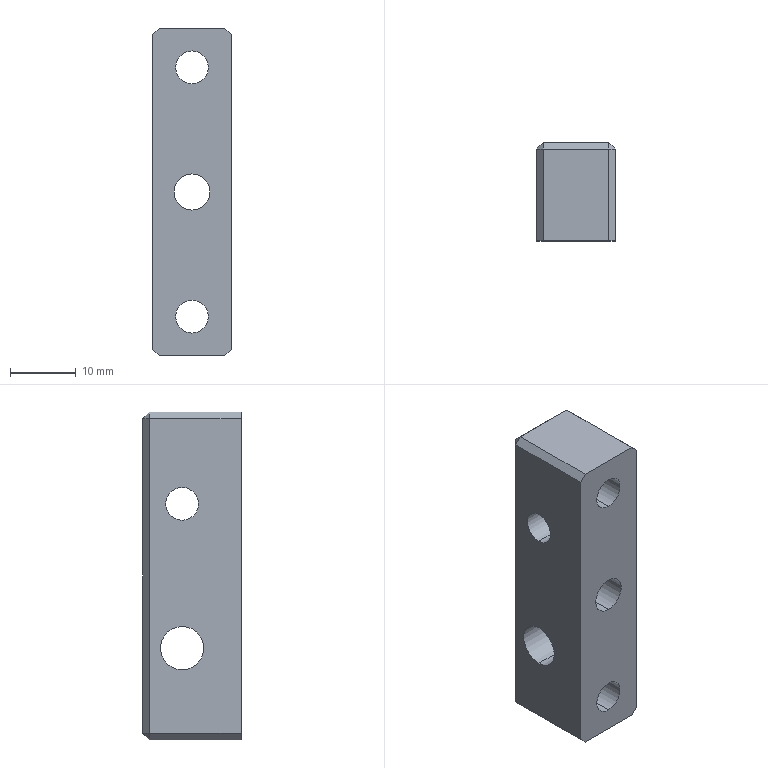Part | SolidWorks | features HoleWzd 3, Chamfer 1, Extrusion 1, ICE 1 | 1 solid | 32 faces | box 12 x 15 x 50 mm | volume 6990 mm3 | plane 20 | cylinder 12 | commonest cylinder face diameters 5 x6 5.5 x2 6.6 x2 10 x2
STEP:
#1=CARTESIAN_POINT('',(0.,9.,-11.5));
#2=VERTEX_POINT('',#1);
#3=CARTESIAN_POINT('',(0.,9.,-16.5));
#4=VERTEX_POINT('',#3);
#5=CARTESIAN_POINT('',(0.,9.,-14.));
#6=DIRECTION('',(1.,0.,0.));
#7=DIRECTION('',(0.,0.,-1.));
#8=AXIS2_PLACEMENT_3D('',#5,#6,#7);
#9=CIRCLE('',#8,2.5);
#10=EDGE_CURVE('',#2,#4,#9,.T.);
#11=ORIENTED_EDGE('',*,*,#10,.F.);
#12=CARTESIAN_POINT('',(12.,9.,-11.5));
#13=VERTEX_POINT('',#12);
#14=CARTESIAN_POINT('',(12.,9.,-11.5));
#15=DIRECTION('',(1.,0.,0.));
#16=VECTOR('',#15,1000.);
#17=LINE('',#14,#16);
#18=EDGE_CURVE('',#2,#13,#17,.T.);
#19=ORIENTED_EDGE('',*,*,#18,.T.);
#20=CARTESIAN_POINT('',(12.,9.,-16.5));
#21=VERTEX_POINT('',#20);
#22=CARTESIAN_POINT('',(12.,9.,-14.));
#23=DIRECTION('',(1.,0.,0.));
#24=DIRECTION('',(0.,0.,-1.));
#25=AXIS2_PLACEMENT_3D('',#22,#23,#24);
#26=CIRCLE('',#25,2.5);
#27=EDGE_CURVE('',#13,#21,#26,.T.);
#28=ORIENTED_EDGE('',*,*,#27,.T.);
#29=CARTESIAN_POINT('',(12.,9.,-16.5));
#30=DIRECTION('',(1.,0.,0.));
#31=VECTOR('',#30,1000.);
#32=LINE('',#29,#31);
#33=EDGE_CURVE('',#4,#21,#32,.T.);
#34=ORIENTED_EDGE('',*,*,#33,.F.);
#35=EDGE_LOOP('',(#11,#19,#28,#34));
#36=FACE_OUTER_BOUND('',#35,.T.);
#37=CARTESIAN_POINT('',(12.,9.,-14.));
#38=DIRECTION('',(1.,0.,0.));
#39=DIRECTION('',(0.,0.,-1.));
#40=AXIS2_PLACEMENT_3D('',#37,#38,#39);
#41=CYLINDRICAL_SURFACE('',#40,2.5);
#42=ADVANCED_FACE('',(#36),#41,.F.);
#43=CARTESIAN_POINT('',(0.,9.,-32.7));
#44=VERTEX_POINT('',#43);
#45=CARTESIAN_POINT('',(0.,9.,-39.3));
#46=VERTEX_POINT('',#45);
#47=CARTESIAN_POINT('',(0.,9.,-36.));
#48=DIRECTION('',(1.,0.,0.));
#49=DIRECTION('',(0.,0.,-1.));
#50=AXIS2_PLACEMENT_3D('',#47,#48,#49);
#51=CIRCLE('',#50,3.3);
#52=EDGE_CURVE('',#44,#46,#51,.T.);
#53=ORIENTED_EDGE('',*,*,#52,.F.);
#54=CARTESIAN_POINT('',(12.,9.,-32.7));
#55=VERTEX_POINT('',#54);
#56=CARTESIAN_POINT('',(12.,9.,-32.7));
#57=DIRECTION('',(1.,0.,0.));
#58=VECTOR('',#57,1000.);
#59=LINE('',#56,#58);
#60=EDGE_CURVE('',#44,#55,#59,.T.);
#61=ORIENTED_EDGE('',*,*,#60,.T.);
#62=CARTESIAN_POINT('',(12.,9.,-39.3));
#63=VERTEX_POINT('',#62);
#64=CARTESIAN_POINT('',(12.,9.,-36.));
#65=DIRECTION('',(1.,0.,0.));
#66=DIRECTION('',(0.,0.,-1.));
#67=AXIS2_PLACEMENT_3D('',#64,#65,#66);
#68=CIRCLE('',#67,3.3);
#69=EDGE_CURVE('',#55,#63,#68,.T.);
#70=ORIENTED_EDGE('',*,*,#69,.T.);
#71=CARTESIAN_POINT('',(12.,9.,-39.3));
#72=DIRECTION('',(1.,0.,0.));
#73=VECTOR('',#72,1000.);
#74=LINE('',#71,#73);
#75=EDGE_CURVE('',#46,#63,#74,.T.);
#76=ORIENTED_EDGE('',*,*,#75,.F.);
#77=EDGE_LOOP('',(#53,#61,#70,#76));
#78=FACE_OUTER_BOUND('',#77,.T.);
#79=CARTESIAN_POINT('',(12.,9.,-36.));
#80=DIRECTION('',(1.,0.,0.));
#81=DIRECTION('',(0.,0.,-1.));
#82=AXIS2_PLACEMENT_3D('',#79,#80,#81);
#83=CYLINDRICAL_SURFACE('',#82,3.3);
#84=ADVANCED_FACE('',(#78),#83,.F.);
#85=CARTESIAN_POINT('',(6.,9.,-30.));
#86=VERTEX_POINT('',#85);
#87=CARTESIAN_POINT('',(6.,9.,-20.));
#88=VERTEX_POINT('',#87);
#89=CARTESIAN_POINT('',(6.,9.,-25.));
#90=DIRECTION('',(0.,1.,0.));
#91=DIRECTION('',(0.,0.,1.));
#92=AXIS2_PLACEMENT_3D('',#89,#90,#91);
#93=CIRCLE('',#92,5.);
#94=EDGE_CURVE('',#86,#88,#93,.T.);
#95=ORIENTED_EDGE('',*,*,#94,.F.);
#96=CARTESIAN_POINT('',(6.,15.,-30.));
#97=VERTEX_POINT('',#96);
#98=CARTESIAN_POINT('',(6.,15.,-30.));
#99=DIRECTION('',(0.,1.,0.));
#100=VECTOR('',#99,1000.);
#101=LINE('',#98,#100);
#102=EDGE_CURVE('',#86,#97,#101,.T.);
#103=ORIENTED_EDGE('',*,*,#102,.T.);
#104=CARTESIAN_POINT('',(1.,15.,-25.));
#105=VERTEX_POINT('',#104);
#106=CARTESIAN_POINT('',(6.,15.,-25.));
#107=DIRECTION('',(0.,1.,0.));
#108=DIRECTION('',(0.,0.,1.));
#109=AXIS2_PLACEMENT_3D('',#106,#107,#108);
#110=CIRCLE('',#109,5.);
#111=EDGE_CURVE('',#97,#105,#110,.T.);
#112=ORIENTED_EDGE('',*,*,#111,.T.);
#113=CARTESIAN_POINT('',(6.,15.,-20.));
#114=VERTEX_POINT('',#113);
#115=CARTESIAN_POINT('',(6.,15.,-25.));
#116=DIRECTION('',(0.,1.,0.));
#117=DIRECTION('',(0.,0.,1.));
#118=AXIS2_PLACEMENT_3D('',#115,#116,#117);
#119=CIRCLE('',#118,5.);
#120=EDGE_CURVE('',#105,#114,#119,.T.);
#121=ORIENTED_EDGE('',*,*,#120,.T.);
#122=CARTESIAN_POINT('',(6.,15.,-20.));
#123=DIRECTION('',(0.,1.,0.));
#124=VECTOR('',#123,1000.);
#125=LINE('',#122,#124);
#126=EDGE_CURVE('',#88,#114,#125,.T.);
#127=ORIENTED_EDGE('',*,*,#126,.F.);
#128=EDGE_LOOP('',(#95,#103,#112,#121,#127));
#129=FACE_OUTER_BOUND('',#128,.T.);
#130=CARTESIAN_POINT('',(6.,15.,-25.));
#131=DIRECTION('',(0.,1.,0.));
#132=DIRECTION('',(0.,0.,1.));
#133=AXIS2_PLACEMENT_3D('',#130,#131,#132);
#134=CYLINDRICAL_SURFACE('',#133,5.);
#135=ADVANCED_FACE('',(#129),#134,.F.);
#136=CARTESIAN_POINT('',(6.,0.,-27.75));
#137=VERTEX_POINT('',#136);
#138=CARTESIAN_POINT('',(6.,0.,-22.25));
#139=VERTEX_POINT('',#138);
#140=CARTESIAN_POINT('',(6.,0.,-25.));
#141=DIRECTION('',(0.,1.,0.));
#142=DIRECTION('',(0.,0.,1.));
#143=AXIS2_PLACEMENT_3D('',#140,#141,#142);
#144=CIRCLE('',#143,2.75);
#145=EDGE_CURVE('',#137,#139,#144,.T.);
#146=ORIENTED_EDGE('',*,*,#145,.F.);
#147=CARTESIAN_POINT('',(6.,9.,-27.75));
#148=VERTEX_POINT('',#147);
#149=CARTESIAN_POINT('',(6.,15.,-27.75));
#150=DIRECTION('',(0.,1.,0.));
#151=VECTOR('',#150,1000.);
#152=LINE('',#149,#151);
#153=EDGE_CURVE('',#137,#148,#152,.T.);
#154=ORIENTED_EDGE('',*,*,#153,.T.);
#155=CARTESIAN_POINT('',(6.,9.,-22.25));
#156=VERTEX_POINT('',#155);
#157=CARTESIAN_POINT('',(6.,9.,-25.));
#158=DIRECTION('',(0.,1.,0.));
#159=DIRECTION('',(0.,0.,1.));
#160=AXIS2_PLACEMENT_3D('',#157,#158,#159);
#161=CIRCLE('',#160,2.75);
#162=EDGE_CURVE('',#148,#156,#161,.T.);
#163=ORIENTED_EDGE('',*,*,#162,.T.);
#164=CARTESIAN_POINT('',(6.,15.,-22.25));
#165=DIRECTION('',(0.,1.,0.));
#166=VECTOR('',#165,1000.);
#167=LINE('',#164,#166);
#168=EDGE_CURVE('',#139,#156,#167,.T.);
#169=ORIENTED_EDGE('',*,*,#168,.F.);
#170=EDGE_LOOP('',(#146,#154,#163,#169));
#171=FACE_OUTER_BOUND('',#170,.T.);
#172=CARTESIAN_POINT('',(6.,15.,-25.));
#173=DIRECTION('',(0.,1.,0.));
#174=DIRECTION('',(0.,0.,1.));
#175=AXIS2_PLACEMENT_3D('',#172,#173,#174);
#176=CYLINDRICAL_SURFACE('',#175,2.75);
#177=ADVANCED_FACE('',(#171),#176,.F.);
#178=CARTESIAN_POINT('',(6.,0.,-8.5));
#179=VERTEX_POINT('',#178);
#180=CARTESIAN_POINT('',(6.,0.,-3.5));
#181=VERTEX_POINT('',#180);
#182=CARTESIAN_POINT('',(6.,0.,-6.));
#183=DIRECTION('',(0.,1.,0.));
#184=DIRECTION('',(0.,0.,1.));
#185=AXIS2_PLACEMENT_3D('',#182,#183,#184);
#186=CIRCLE('',#185,2.5);
#187=EDGE_CURVE('',#179,#181,#186,.T.);
#188=ORIENTED_EDGE('',*,*,#187,.F.);
#189=CARTESIAN_POINT('',(6.,15.,-8.5));
#190=VERTEX_POINT('',#189);
#191=CARTESIAN_POINT('',(6.,0.,-8.5));
#192=DIRECTION('',(0.,1.,0.));
#193=VECTOR('',#192,1000.);
#194=LINE('',#191,#193);
#195=EDGE_CURVE('',#179,#190,#194,.T.);
#196=ORIENTED_EDGE('',*,*,#195,.T.);
#197=CARTESIAN_POINT('',(6.,15.,-3.5));
#198=VERTEX_POINT('',#197);
#199=CARTESIAN_POINT('',(6.,15.,-6.));
#200=DIRECTION('',(0.,1.,0.));
#201=DIRECTION('',(0.,0.,1.));
#202=AXIS2_PLACEMENT_3D('',#199,#200,#201);
#203=CIRCLE('',#202,2.5);
#204=EDGE_CURVE('',#190,#198,#203,.T.);
#205=ORIENTED_EDGE('',*,*,#204,.T.);
#206=CARTESIAN_POINT('',(6.,0.,-3.5));
#207=DIRECTION('',(0.,1.,0.));
#208=VECTOR('',#207,1000.);
#209=LINE('',#206,#208);
#210=EDGE_CURVE('',#181,#198,#209,.T.);
#211=ORIENTED_EDGE('',*,*,#210,.F.);
#212=EDGE_LOOP('',(#188,#196,#205,#211));
#213=FACE_OUTER_BOUND('',#212,.T.);
#214=CARTESIAN_POINT('',(6.,0.,-6.));
#215=DIRECTION('',(0.,1.,0.));
#216=DIRECTION('',(0.,0.,1.));
#217=AXIS2_PLACEMENT_3D('',#214,#215,#216);
#218=CYLINDRICAL_SURFACE('',#217,2.5);
#219=ADVANCED_FACE('',(#213),#218,.F.);
#220=CARTESIAN_POINT('',(6.,0.,-46.5));
#221=VERTEX_POINT('',#220);
#222=CARTESIAN_POINT('',(6.,0.,-41.5));
#223=VERTEX_POINT('',#222);
#224=CARTESIAN_POINT('',(6.,0.,-44.));
#225=DIRECTION('',(0.,1.,0.));
#226=DIRECTION('',(0.,0.,1.));
#227=AXIS2_PLACEMENT_3D('',#224,#225,#226);
#228=CIRCLE('',#227,2.5);
#229=EDGE_CURVE('',#221,#223,#228,.T.);
#230=ORIENTED_EDGE('',*,*,#229,.F.);
#231=CARTESIAN_POINT('',(6.,15.,-46.5));
#232=VERTEX_POINT('',#231);
#233=CARTESIAN_POINT('',(6.,0.,-46.5));
#234=DIRECTION('',(0.,1.,0.));
#235=VECTOR('',#234,1000.);
#236=LINE('',#233,#235);
#237=EDGE_CURVE('',#221,#232,#236,.T.);
#238=ORIENTED_EDGE('',*,*,#237,.T.);
#239=CARTESIAN_POINT('',(6.,15.,-41.5));
#240=VERTEX_POINT('',#239);
#241=CARTESIAN_POINT('',(6.,15.,-44.));
#242=DIRECTION('',(0.,1.,0.));
#243=DIRECTION('',(0.,0.,1.));
#244=AXIS2_PLACEMENT_3D('',#241,#242,#243);
#245=CIRCLE('',#244,2.5);
#246=EDGE_CURVE('',#232,#240,#245,.T.);
#247=ORIENTED_EDGE('',*,*,#246,.T.);
#248=CARTESIAN_POINT('',(6.,0.,-41.5));
#249=DIRECTION('',(0.,1.,0.));
#250=VECTOR('',#249,1000.);
#251=LINE('',#248,#250);
#252=EDGE_CURVE('',#223,#240,#251,.T.);
#253=ORIENTED_EDGE('',*,*,#252,.F.);
#254=EDGE_LOOP('',(#230,#238,#247,#253));
#255=FACE_OUTER_BOUND('',#254,.T.);
#256=CARTESIAN_POINT('',(6.,0.,-44.));
#257=DIRECTION('',(0.,1.,0.));
#258=DIRECTION('',(0.,0.,1.));
#259=AXIS2_PLACEMENT_3D('',#256,#257,#258);
#260=CYLINDRICAL_SURFACE('',#259,2.5);
#261=ADVANCED_FACE('',(#255),#260,.F.);
#262=CARTESIAN_POINT('',(6.,15.,-44.));
#263=DIRECTION('',(0.,1.,0.));
#264=DIRECTION('',(0.,0.,1.));
#265=AXIS2_PLACEMENT_3D('',#262,#263,#264);
#266=CIRCLE('',#265,2.5);
#267=EDGE_CURVE('',#240,#232,#266,.T.);
#268=ORIENTED_EDGE('',*,*,#267,.F.);
#269=ORIENTED_EDGE('',*,*,#246,.F.);
#270=EDGE_LOOP('',(#268,#269));
#271=FACE_BOUND('',#270,.T.);
#272=CARTESIAN_POINT('',(11.,15.,-25.));
#273=VERTEX_POINT('',#272);
#274=CARTESIAN_POINT('',(11.,15.,-49.));
#275=VERTEX_POINT('',#274);
#276=CARTESIAN_POINT('',(11.,15.,0.));
#277=DIRECTION('',(0.,0.,-1.));
#278=VECTOR('',#277,1000.);
#279=LINE('',#276,#278);
#280=EDGE_CURVE('',#273,#275,#279,.T.);
#281=ORIENTED_EDGE('',*,*,#280,.T.);
#282=CARTESIAN_POINT('',(1.,15.,-49.));
#283=VERTEX_POINT('',#282);
#284=CARTESIAN_POINT('',(0.,15.,-49.));
#285=DIRECTION('',(-1.,0.,0.));
#286=VECTOR('',#285,1000.);
#287=LINE('',#284,#286);
#288=EDGE_CURVE('',#275,#283,#287,.T.);
#289=ORIENTED_EDGE('',*,*,#288,.T.);
#290=CARTESIAN_POINT('',(1.,15.,0.));
#291=DIRECTION('',(0.,0.,1.));
#292=VECTOR('',#291,1000.);
#293=LINE('',#290,#292);
#294=EDGE_CURVE('',#283,#105,#293,.T.);
#295=ORIENTED_EDGE('',*,*,#294,.T.);
#296=ORIENTED_EDGE('',*,*,#111,.F.);
#297=CARTESIAN_POINT('',(6.,15.,-25.));
#298=DIRECTION('',(0.,1.,0.));
#299=DIRECTION('',(0.,0.,1.));
#300=AXIS2_PLACEMENT_3D('',#297,#298,#299);
#301=CIRCLE('',#300,5.);
#302=EDGE_CURVE('',#273,#97,#301,.T.);
#303=ORIENTED_EDGE('',*,*,#302,.F.);
#304=EDGE_LOOP('',(#281,#289,#295,#296,#303));
#305=FACE_OUTER_BOUND('',#304,.T.);
#306=CARTESIAN_POINT('',(0.,15.,0.));
#307=DIRECTION('',(0.,-1.,0.));
#308=DIRECTION('',(0.,0.,-1.));
#309=AXIS2_PLACEMENT_3D('',#306,#307,#308);
#310=PLANE('',#309);
#311=ADVANCED_FACE('',(#271,#305),#310,.F.);
#312=CARTESIAN_POINT('',(0.,9.,-14.));
#313=DIRECTION('',(1.,0.,0.));
#314=DIRECTION('',(0.,0.,-1.));
#315=AXIS2_PLACEMENT_3D('',#312,#313,#314);
#316=CIRCLE('',#315,2.5);
#317=EDGE_CURVE('',#4,#2,#316,.T.);
#318=ORIENTED_EDGE('',*,*,#317,.T.);
#319=ORIENTED_EDGE('',*,*,#10,.T.);
#320=EDGE_LOOP('',(#318,#319));
#321=FACE_BOUND('',#320,.T.);
#322=CARTESIAN_POINT('',(0.,9.,-36.));
#323=DIRECTION('',(1.,0.,0.));
#324=DIRECTION('',(0.,0.,-1.));
#325=AXIS2_PLACEMENT_3D('',#322,#323,#324);
#326=CIRCLE('',#325,3.3);
#327=EDGE_CURVE('',#46,#44,#326,.T.);
#328=ORIENTED_EDGE('',*,*,#327,.T.);
#329=ORIENTED_EDGE('',*,*,#52,.T.);
#330=EDGE_LOOP('',(#328,#329));
#331=FACE_BOUND('',#330,.T.);
#332=CARTESIAN_POINT('',(0.,14.,-1.));
#333=VERTEX_POINT('',#332);
#334=CARTESIAN_POINT('',(0.,14.,-49.));
#335=VERTEX_POINT('',#334);
#336=CARTESIAN_POINT('',(0.,14.,0.));
#337=DIRECTION('',(0.,0.,-1.));
#338=VECTOR('',#337,1000.);
#339=LINE('',#336,#338);
#340=EDGE_CURVE('',#333,#335,#339,.T.);
#341=ORIENTED_EDGE('',*,*,#340,.T.);
#342=CARTESIAN_POINT('',(0.,0.,-49.));
#343=VERTEX_POINT('',#342);
#344=CARTESIAN_POINT('',(0.,15.,-49.));
#345=DIRECTION('',(0.,-1.,0.));
#346=VECTOR('',#345,1000.);
#347=LINE('',#344,#346);
#348=EDGE_CURVE('',#335,#343,#347,.T.);
#349=ORIENTED_EDGE('',*,*,#348,.T.);
#350=CARTESIAN_POINT('',(0.,0.,-1.));
#351=VERTEX_POINT('',#350);
#352=CARTESIAN_POINT('',(0.,0.,0.));
#353=DIRECTION('',(0.,0.,1.));
#354=VECTOR('',#353,1000.);
#355=LINE('',#352,#354);
#356=EDGE_CURVE('',#343,#351,#355,.T.);
#357=ORIENTED_EDGE('',*,*,#356,.T.);
#358=CARTESIAN_POINT('',(0.,15.,-1.));
#359=DIRECTION('',(0.,1.,0.));
#360=VECTOR('',#359,1000.);
#361=LINE('',#358,#360);
#362=EDGE_CURVE('',#351,#333,#361,.T.);
#363=ORIENTED_EDGE('',*,*,#362,.T.);
#364=EDGE_LOOP('',(#341,#349,#357,#363));
#365=FACE_OUTER_BOUND('',#364,.T.);
#366=CARTESIAN_POINT('',(0.,15.,0.));
#367=DIRECTION('',(1.,0.,0.));
#368=DIRECTION('',(0.,0.,-1.));
#369=AXIS2_PLACEMENT_3D('',#366,#367,#368);
#370=PLANE('',#369);
#371=ADVANCED_FACE('',(#321,#331,#365),#370,.F.);
#372=CARTESIAN_POINT('',(11.,14.,0.));
#373=VERTEX_POINT('',#372);
#374=CARTESIAN_POINT('',(1.,14.,0.));
#375=VERTEX_POINT('',#374);
#376=CARTESIAN_POINT('',(0.,14.,0.));
#377=DIRECTION('',(-1.,0.,0.));
#378=VECTOR('',#377,1000.);
#379=LINE('',#376,#378);
#380=EDGE_CURVE('',#373,#375,#379,.T.);
#381=ORIENTED_EDGE('',*,*,#380,.T.);
#382=CARTESIAN_POINT('',(1.,0.,0.));
#383=VERTEX_POINT('',#382);
#384=CARTESIAN_POINT('',(1.,15.,0.));
#385=DIRECTION('',(0.,-1.,0.));
#386=VECTOR('',#385,1000.);
#387=LINE('',#384,#386);
#388=EDGE_CURVE('',#375,#383,#387,.T.);
#389=ORIENTED_EDGE('',*,*,#388,.T.);
#390=CARTESIAN_POINT('',(11.,0.,0.));
#391=VERTEX_POINT('',#390);
#392=CARTESIAN_POINT('',(0.,0.,0.));
#393=DIRECTION('',(1.,0.,0.));
#394=VECTOR('',#393,1000.);
#395=LINE('',#392,#394);
#396=EDGE_CURVE('',#383,#391,#395,.T.);
#397=ORIENTED_EDGE('',*,*,#396,.T.);
#398=CARTESIAN_POINT('',(11.,15.,0.));
#399=DIRECTION('',(0.,1.,0.));
#400=VECTOR('',#399,1000.);
#401=LINE('',#398,#400);
#402=EDGE_CURVE('',#391,#373,#401,.T.);
#403=ORIENTED_EDGE('',*,*,#402,.T.);
#404=EDGE_LOOP('',(#381,#389,#397,#403));
#405=FACE_OUTER_BOUND('',#404,.T.);
#406=CARTESIAN_POINT('',(0.,15.,0.));
#407=DIRECTION('',(0.,0.,-1.));
#408=DIRECTION('',(-1.,0.,0.));
#409=AXIS2_PLACEMENT_3D('',#406,#407,#408);
#410=PLANE('',#409);
#411=ADVANCED_FACE('',(#405),#410,.F.);
#412=CARTESIAN_POINT('',(12.,9.,-14.));
#413=DIRECTION('',(1.,0.,0.));
#414=DIRECTION('',(0.,0.,-1.));
#415=AXIS2_PLACEMENT_3D('',#412,#413,#414);
#416=CIRCLE('',#415,2.5);
#417=EDGE_CURVE('',#21,#13,#416,.T.);
#418=ORIENTED_EDGE('',*,*,#417,.F.);
#419=ORIENTED_EDGE('',*,*,#27,.F.);
#420=EDGE_LOOP('',(#418,#419));
#421=FACE_BOUND('',#420,.T.);
#422=CARTESIAN_POINT('',(12.,9.,-36.));
#423=DIRECTION('',(1.,0.,0.));
#424=DIRECTION('',(0.,0.,-1.));
#425=AXIS2_PLACEMENT_3D('',#422,#423,#424);
#426=CIRCLE('',#425,3.3);
#427=EDGE_CURVE('',#63,#55,#426,.T.);
#428=ORIENTED_EDGE('',*,*,#427,.F.);
#429=ORIENTED_EDGE('',*,*,#69,.F.);
#430=EDGE_LOOP('',(#428,#429));
#431=FACE_BOUND('',#430,.T.);
#432=CARTESIAN_POINT('',(12.,0.,-1.));
#433=VERTEX_POINT('',#432);
#434=CARTESIAN_POINT('',(12.,0.,-49.));
#435=VERTEX_POINT('',#434);
#436=CARTESIAN_POINT('',(12.,0.,0.));
#437=DIRECTION('',(0.,0.,-1.));
#438=VECTOR('',#437,1000.);
#439=LINE('',#436,#438);
#440=EDGE_CURVE('',#433,#435,#439,.T.);
#441=ORIENTED_EDGE('',*,*,#440,.T.);
#442=CARTESIAN_POINT('',(12.,14.,-49.));
#443=VERTEX_POINT('',#442);
#444=CARTESIAN_POINT('',(12.,15.,-49.));
#445=DIRECTION('',(0.,1.,0.));
#446=VECTOR('',#445,1000.);
#447=LINE('',#444,#446);
#448=EDGE_CURVE('',#435,#443,#447,.T.);
#449=ORIENTED_EDGE('',*,*,#448,.T.);
#450=CARTESIAN_POINT('',(12.,14.,-1.));
#451=VERTEX_POINT('',#450);
#452=CARTESIAN_POINT('',(12.,14.,0.));
#453=DIRECTION('',(0.,0.,1.));
#454=VECTOR('',#453,1000.);
#455=LINE('',#452,#454);
#456=EDGE_CURVE('',#443,#451,#455,.T.);
#457=ORIENTED_EDGE('',*,*,#456,.T.);
#458=CARTESIAN_POINT('',(12.,15.,-1.));
#459=DIRECTION('',(0.,-1.,0.));
#460=VECTOR('',#459,1000.);
#461=LINE('',#458,#460);
#462=EDGE_CURVE('',#451,#433,#461,.T.);
#463=ORIENTED_EDGE('',*,*,#462,.T.);
#464=EDGE_LOOP('',(#441,#449,#457,#463));
#465=FACE_OUTER_BOUND('',#464,.T.);
#466=CARTESIAN_POINT('',(12.,15.,0.));
#467=DIRECTION('',(-1.,0.,0.));
#468=DIRECTION('',(0.,0.,1.));
#469=AXIS2_PLACEMENT_3D('',#466,#467,#468);
#470=PLANE('',#469);
#471=ADVANCED_FACE('',(#421,#431,#465),#470,.F.);
#472=CARTESIAN_POINT('',(11.,0.,-50.));
#473=VERTEX_POINT('',#472);
#474=CARTESIAN_POINT('',(1.,0.,-50.));
#475=VERTEX_POINT('',#474);
#476=CARTESIAN_POINT('',(0.,0.,-50.));
#477=DIRECTION('',(-1.,0.,0.));
#478=VECTOR('',#477,1000.);
#479=LINE('',#476,#478);
#480=EDGE_CURVE('',#473,#475,#479,.T.);
#481=ORIENTED_EDGE('',*,*,#480,.T.);
#482=CARTESIAN_POINT('',(1.,14.,-50.));
#483=VERTEX_POINT('',#482);
#484=CARTESIAN_POINT('',(1.,15.,-50.));
#485=DIRECTION('',(0.,1.,0.));
#486=VECTOR('',#485,1000.);
#487=LINE('',#484,#486);
#488=EDGE_CURVE('',#475,#483,#487,.T.);
#489=ORIENTED_EDGE('',*,*,#488,.T.);
#490=CARTESIAN_POINT('',(11.,14.,-50.));
#491=VERTEX_POINT('',#490);
#492=CARTESIAN_POINT('',(0.,14.,-50.));
#493=DIRECTION('',(1.,0.,0.));
#494=VECTOR('',#493,1000.);
#495=LINE('',#492,#494);
#496=EDGE_CURVE('',#483,#491,#495,.T.);
#497=ORIENTED_EDGE('',*,*,#496,.T.);
#498=CARTESIAN_POINT('',(11.,15.,-50.));
#499=DIRECTION('',(0.,-1.,0.));
#500=VECTOR('',#499,1000.);
#501=LINE('',#498,#500);
#502=EDGE_CURVE('',#491,#473,#501,.T.);
#503=ORIENTED_EDGE('',*,*,#502,.T.);
#504=EDGE_LOOP('',(#481,#489,#497,#503));
#505=FACE_OUTER_BOUND('',#504,.T.);
#506=CARTESIAN_POINT('',(0.,15.,-50.));
#507=DIRECTION('',(0.,0.,1.));
#508=DIRECTION('',(1.,0.,0.));
#509=AXIS2_PLACEMENT_3D('',#506,#507,#508);
#510=PLANE('',#509);
#511=ADVANCED_FACE('',(#505),#510,.F.);
#512=ORIENTED_EDGE('',*,*,#120,.F.);
#513=CARTESIAN_POINT('',(1.,15.,-1.));
#514=VERTEX_POINT('',#513);
#515=CARTESIAN_POINT('',(1.,15.,0.));
#516=DIRECTION('',(0.,0.,1.));
#517=VECTOR('',#516,1000.);
#518=LINE('',#515,#517);
#519=EDGE_CURVE('',#105,#514,#518,.T.);
#520=ORIENTED_EDGE('',*,*,#519,.T.);
#521=CARTESIAN_POINT('',(11.,15.,-1.));
#522=VERTEX_POINT('',#521);
#523=CARTESIAN_POINT('',(0.,15.,-1.));
#524=DIRECTION('',(1.,0.,0.));
#525=VECTOR('',#524,1000.);
#526=LINE('',#523,#525);
#527=EDGE_CURVE('',#514,#522,#526,.T.);
#528=ORIENTED_EDGE('',*,*,#527,.T.);
#529=CARTESIAN_POINT('',(11.,15.,0.));
#530=DIRECTION('',(0.,0.,-1.));
#531=VECTOR('',#530,1000.);
#532=LINE('',#529,#531);
#533=EDGE_CURVE('',#522,#273,#532,.T.);
#534=ORIENTED_EDGE('',*,*,#533,.T.);
#535=CARTESIAN_POINT('',(6.,15.,-25.));
#536=DIRECTION('',(0.,1.,0.));
#537=DIRECTION('',(0.,0.,1.));
#538=AXIS2_PLACEMENT_3D('',#535,#536,#537);
#539=CIRCLE('',#538,5.);
#540=EDGE_CURVE('',#114,#273,#539,.T.);
#541=ORIENTED_EDGE('',*,*,#540,.F.);
#542=EDGE_LOOP('',(#512,#520,#528,#534,#541));
#543=FACE_OUTER_BOUND('',#542,.T.);
#544=CARTESIAN_POINT('',(6.,15.,-6.));
#545=DIRECTION('',(0.,1.,0.));
#546=DIRECTION('',(0.,0.,1.));
#547=AXIS2_PLACEMENT_3D('',#544,#545,#546);
#548=CIRCLE('',#547,2.5);
#549=EDGE_CURVE('',#198,#190,#548,.T.);
#550=ORIENTED_EDGE('',*,*,#549,.F.);
#551=ORIENTED_EDGE('',*,*,#204,.F.);
#552=EDGE_LOOP('',(#550,#551));
#553=FACE_BOUND('',#552,.T.);
#554=CARTESIAN_POINT('',(0.,15.,0.));
#555=DIRECTION('',(0.,-1.,0.));
#556=DIRECTION('',(0.,0.,-1.));
#557=AXIS2_PLACEMENT_3D('',#554,#555,#556);
#558=PLANE('',#557);
#559=ADVANCED_FACE('',(#543,#553),#558,.F.);
#560=CARTESIAN_POINT('',(6.,0.,-25.));
#561=DIRECTION('',(0.,1.,0.));
#562=DIRECTION('',(0.,0.,1.));
#563=AXIS2_PLACEMENT_3D('',#560,#561,#562);
#564=CIRCLE('',#563,2.75);
#565=EDGE_CURVE('',#139,#137,#564,.T.);
#566=ORIENTED_EDGE('',*,*,#565,.T.);
#567=ORIENTED_EDGE('',*,*,#145,.T.);
#568=EDGE_LOOP('',(#566,#567));
#569=FACE_BOUND('',#568,.T.);
#570=CARTESIAN_POINT('',(6.,0.,-6.));
#571=DIRECTION('',(0.,1.,0.));
#572=DIRECTION('',(0.,0.,1.));
#573=AXIS2_PLACEMENT_3D('',#570,#571,#572);
#574=CIRCLE('',#573,2.5);
#575=EDGE_CURVE('',#181,#179,#574,.T.);
#576=ORIENTED_EDGE('',*,*,#575,.T.);
#577=ORIENTED_EDGE('',*,*,#187,.T.);
#578=EDGE_LOOP('',(#576,#577));
#579=FACE_BOUND('',#578,.T.);
#580=CARTESIAN_POINT('',(6.,0.,-44.));
#581=DIRECTION('',(0.,1.,0.));
#582=DIRECTION('',(0.,0.,1.));
#583=AXIS2_PLACEMENT_3D('',#580,#581,#582);
#584=CIRCLE('',#583,2.5);
#585=EDGE_CURVE('',#223,#221,#584,.T.);
#586=ORIENTED_EDGE('',*,*,#585,.T.);
#587=ORIENTED_EDGE('',*,*,#229,.T.);
#588=EDGE_LOOP('',(#586,#587));
#589=FACE_BOUND('',#588,.T.);
#590=ORIENTED_EDGE('',*,*,#356,.F.);
#591=CARTESIAN_POINT('',(-24.5,0.,-24.5));
#592=DIRECTION('',(0.7071,0.,-0.7071));
#593=VECTOR('',#592,1000.);
#594=LINE('',#591,#593);
#595=EDGE_CURVE('',#343,#475,#594,.T.);
#596=ORIENTED_EDGE('',*,*,#595,.T.);
#597=ORIENTED_EDGE('',*,*,#480,.F.);
#598=CARTESIAN_POINT('',(30.5,0.,-30.5));
#599=DIRECTION('',(0.7071,0.,0.7071));
#600=VECTOR('',#599,1000.);
#601=LINE('',#598,#600);
#602=EDGE_CURVE('',#473,#435,#601,.T.);
#603=ORIENTED_EDGE('',*,*,#602,.T.);
#604=ORIENTED_EDGE('',*,*,#440,.F.);
#605=CARTESIAN_POINT('',(5.5,0.,5.5));
#606=DIRECTION('',(-0.7071,0.,0.7071));
#607=VECTOR('',#606,1000.);
#608=LINE('',#605,#607);
#609=EDGE_CURVE('',#433,#391,#608,.T.);
#610=ORIENTED_EDGE('',*,*,#609,.T.);
#611=ORIENTED_EDGE('',*,*,#396,.F.);
#612=CARTESIAN_POINT('',(0.5,0.,-0.5));
#613=DIRECTION('',(-0.7071,0.,-0.7071));
#614=VECTOR('',#613,1000.);
#615=LINE('',#612,#614);
#616=EDGE_CURVE('',#383,#351,#615,.T.);
#617=ORIENTED_EDGE('',*,*,#616,.T.);
#618=EDGE_LOOP('',(#590,#596,#597,#603,#604,#610,#611,#617));
#619=FACE_OUTER_BOUND('',#618,.T.);
#620=CARTESIAN_POINT('',(0.,0.,0.));
#621=DIRECTION('',(0.,-1.,0.));
#622=DIRECTION('',(0.,0.,-1.));
#623=AXIS2_PLACEMENT_3D('',#620,#621,#622);
#624=PLANE('',#623);
#625=ADVANCED_FACE('',(#569,#579,#589,#619),#624,.T.);
#626=ORIENTED_EDGE('',*,*,#237,.F.);
#627=ORIENTED_EDGE('',*,*,#585,.F.);
#628=ORIENTED_EDGE('',*,*,#252,.T.);
#629=ORIENTED_EDGE('',*,*,#267,.T.);
#630=EDGE_LOOP('',(#626,#627,#628,#629));
#631=FACE_OUTER_BOUND('',#630,.T.);
#632=CARTESIAN_POINT('',(6.,0.,-44.));
#633=DIRECTION('',(0.,1.,0.));
#634=DIRECTION('',(0.,0.,1.));
#635=AXIS2_PLACEMENT_3D('',#632,#633,#634);
#636=CYLINDRICAL_SURFACE('',#635,2.5);
#637=ADVANCED_FACE('',(#631),#636,.F.);
#638=ORIENTED_EDGE('',*,*,#195,.F.);
#639=ORIENTED_EDGE('',*,*,#575,.F.);
#640=ORIENTED_EDGE('',*,*,#210,.T.);
#641=ORIENTED_EDGE('',*,*,#549,.T.);
#642=EDGE_LOOP('',(#638,#639,#640,#641));
#643=FACE_OUTER_BOUND('',#642,.T.);
#644=CARTESIAN_POINT('',(6.,0.,-6.));
#645=DIRECTION('',(0.,1.,0.));
#646=DIRECTION('',(0.,0.,1.));
#647=AXIS2_PLACEMENT_3D('',#644,#645,#646);
#648=CYLINDRICAL_SURFACE('',#647,2.5);
#649=ADVANCED_FACE('',(#643),#648,.F.);
#650=ORIENTED_EDGE('',*,*,#153,.F.);
#651=ORIENTED_EDGE('',*,*,#565,.F.);
#652=ORIENTED_EDGE('',*,*,#168,.T.);
#653=CARTESIAN_POINT('',(6.,9.,-25.));
#654=DIRECTION('',(0.,1.,0.));
#655=DIRECTION('',(0.,0.,1.));
#656=AXIS2_PLACEMENT_3D('',#653,#654,#655);
#657=CIRCLE('',#656,2.75);
#658=EDGE_CURVE('',#156,#148,#657,.T.);
#659=ORIENTED_EDGE('',*,*,#658,.T.);
#660=EDGE_LOOP('',(#650,#651,#652,#659));
#661=FACE_OUTER_BOUND('',#660,.T.);
#662=CARTESIAN_POINT('',(6.,15.,-25.));
#663=DIRECTION('',(0.,1.,0.));
#664=DIRECTION('',(0.,0.,1.));
#665=AXIS2_PLACEMENT_3D('',#662,#663,#664);
#666=CYLINDRICAL_SURFACE('',#665,2.75);
#667=ADVANCED_FACE('',(#661),#666,.F.);
#668=ORIENTED_EDGE('',*,*,#658,.F.);
#669=ORIENTED_EDGE('',*,*,#162,.F.);
#670=EDGE_LOOP('',(#668,#669));
#671=FACE_BOUND('',#670,.T.);
#672=CARTESIAN_POINT('',(6.,9.,-25.));
#673=DIRECTION('',(0.,1.,0.));
#674=DIRECTION('',(0.,0.,1.));
#675=AXIS2_PLACEMENT_3D('',#672,#673,#674);
#676=CIRCLE('',#675,5.);
#677=EDGE_CURVE('',#88,#86,#676,.T.);
#678=ORIENTED_EDGE('',*,*,#677,.T.);
#679=ORIENTED_EDGE('',*,*,#94,.T.);
#680=EDGE_LOOP('',(#678,#679));
#681=FACE_OUTER_BOUND('',#680,.T.);
#682=CARTESIAN_POINT('',(8.75,9.,-25.));
#683=DIRECTION('',(0.,-1.,0.));
#684=DIRECTION('',(0.,0.,-1.));
#685=AXIS2_PLACEMENT_3D('',#682,#683,#684);
#686=PLANE('',#685);
#687=ADVANCED_FACE('',(#671,#681),#686,.F.);
#688=ORIENTED_EDGE('',*,*,#102,.F.);
#689=ORIENTED_EDGE('',*,*,#677,.F.);
#690=ORIENTED_EDGE('',*,*,#126,.T.);
#691=ORIENTED_EDGE('',*,*,#540,.T.);
#692=ORIENTED_EDGE('',*,*,#302,.T.);
#693=EDGE_LOOP('',(#688,#689,#690,#691,#692));
#694=FACE_OUTER_BOUND('',#693,.T.);
#695=CARTESIAN_POINT('',(6.,15.,-25.));
#696=DIRECTION('',(0.,1.,0.));
#697=DIRECTION('',(0.,0.,1.));
#698=AXIS2_PLACEMENT_3D('',#695,#696,#697);
#699=CYLINDRICAL_SURFACE('',#698,5.);
#700=ADVANCED_FACE('',(#694),#699,.F.);
#701=ORIENTED_EDGE('',*,*,#60,.F.);
#702=ORIENTED_EDGE('',*,*,#327,.F.);
#703=ORIENTED_EDGE('',*,*,#75,.T.);
#704=ORIENTED_EDGE('',*,*,#427,.T.);
#705=EDGE_LOOP('',(#701,#702,#703,#704));
#706=FACE_OUTER_BOUND('',#705,.T.);
#707=CARTESIAN_POINT('',(12.,9.,-36.));
#708=DIRECTION('',(1.,0.,0.));
#709=DIRECTION('',(0.,0.,-1.));
#710=AXIS2_PLACEMENT_3D('',#707,#708,#709);
#711=CYLINDRICAL_SURFACE('',#710,3.3);
#712=ADVANCED_FACE('',(#706),#711,.F.);
#713=ORIENTED_EDGE('',*,*,#18,.F.);
#714=ORIENTED_EDGE('',*,*,#317,.F.);
#715=ORIENTED_EDGE('',*,*,#33,.T.);
#716=ORIENTED_EDGE('',*,*,#417,.T.);
#717=EDGE_LOOP('',(#713,#714,#715,#716));
#718=FACE_OUTER_BOUND('',#717,.T.);
#719=CARTESIAN_POINT('',(12.,9.,-14.));
#720=DIRECTION('',(1.,0.,0.));
#721=DIRECTION('',(0.,0.,-1.));
#722=AXIS2_PLACEMENT_3D('',#719,#720,#721);
#723=CYLINDRICAL_SURFACE('',#722,2.5);
#724=ADVANCED_FACE('',(#718),#723,.F.);
#725=ORIENTED_EDGE('',*,*,#602,.F.);
#726=ORIENTED_EDGE('',*,*,#502,.F.);
#727=CARTESIAN_POINT('',(12.,14.,-49.));
#728=DIRECTION('',(-0.7071,0.,-0.7071));
#729=VECTOR('',#728,1000.);
#730=LINE('',#727,#729);
#731=EDGE_CURVE('',#443,#491,#730,.T.);
#732=ORIENTED_EDGE('',*,*,#731,.F.);
#733=ORIENTED_EDGE('',*,*,#448,.F.);
#734=EDGE_LOOP('',(#725,#726,#732,#733));
#735=FACE_OUTER_BOUND('',#734,.T.);
#736=CARTESIAN_POINT('',(11.,15.,-50.));
#737=DIRECTION('',(-0.7071,0.,0.7071));
#738=DIRECTION('',(0.,-1.,0.));
#739=AXIS2_PLACEMENT_3D('',#736,#737,#738);
#740=PLANE('',#739);
#741=ADVANCED_FACE('',(#735),#740,.F.);
#742=CARTESIAN_POINT('',(12.,14.,-1.));
#743=DIRECTION('',(-0.7071,0.7071,0.));
#744=VECTOR('',#743,1000.);
#745=LINE('',#742,#744);
#746=EDGE_CURVE('',#451,#522,#745,.T.);
#747=ORIENTED_EDGE('',*,*,#746,.F.);
#748=ORIENTED_EDGE('',*,*,#456,.F.);
#749=CARTESIAN_POINT('',(12.,14.,-49.));
#750=DIRECTION('',(0.7071,-0.7071,0.));
#751=VECTOR('',#750,1000.);
#752=LINE('',#749,#751);
#753=EDGE_CURVE('',#275,#443,#752,.T.);
#754=ORIENTED_EDGE('',*,*,#753,.F.);
#755=ORIENTED_EDGE('',*,*,#280,.F.);
#756=ORIENTED_EDGE('',*,*,#533,.F.);
#757=EDGE_LOOP('',(#747,#748,#754,#755,#756));
#758=FACE_OUTER_BOUND('',#757,.T.);
#759=CARTESIAN_POINT('',(11.,15.,0.));
#760=DIRECTION('',(-0.7071,-0.7071,0.));
#761=DIRECTION('',(0.,0.,-1.));
#762=AXIS2_PLACEMENT_3D('',#759,#760,#761);
#763=PLANE('',#762);
#764=ADVANCED_FACE('',(#758),#763,.F.);
#765=ORIENTED_EDGE('',*,*,#609,.F.);
#766=ORIENTED_EDGE('',*,*,#462,.F.);
#767=CARTESIAN_POINT('',(12.,14.,-1.));
#768=DIRECTION('',(0.7071,0.,-0.7071));
#769=VECTOR('',#768,1000.);
#770=LINE('',#767,#769);
#771=EDGE_CURVE('',#373,#451,#770,.T.);
#772=ORIENTED_EDGE('',*,*,#771,.F.);
#773=ORIENTED_EDGE('',*,*,#402,.F.);
#774=EDGE_LOOP('',(#765,#766,#772,#773));
#775=FACE_OUTER_BOUND('',#774,.T.);
#776=CARTESIAN_POINT('',(12.,15.,-1.));
#777=DIRECTION('',(-0.7071,0.,-0.7071));
#778=DIRECTION('',(0.,-1.,0.));
#779=AXIS2_PLACEMENT_3D('',#776,#777,#778);
#780=PLANE('',#779);
#781=ADVANCED_FACE('',(#775),#780,.F.);
#782=ORIENTED_EDGE('',*,*,#753,.T.);
#783=ORIENTED_EDGE('',*,*,#731,.T.);
#784=CARTESIAN_POINT('',(11.,14.5,-49.5));
#785=DIRECTION('',(0.,-0.7071,-0.7071));
#786=VECTOR('',#785,1000.);
#787=LINE('',#784,#786);
#788=EDGE_CURVE('',#275,#491,#787,.T.);
#789=ORIENTED_EDGE('',*,*,#788,.F.);
#790=EDGE_LOOP('',(#782,#783,#789));
#791=FACE_OUTER_BOUND('',#790,.T.);
#792=CARTESIAN_POINT('',(12.,14.,-49.));
#793=DIRECTION('',(0.5774,0.5774,-0.5774));
#794=DIRECTION('',(-0.7071,0.,-0.7071));
#795=AXIS2_PLACEMENT_3D('',#792,#793,#794);
#796=PLANE('',#795);
#797=ADVANCED_FACE('',(#791),#796,.T.);
#798=ORIENTED_EDGE('',*,*,#771,.T.);
#799=ORIENTED_EDGE('',*,*,#746,.T.);
#800=CARTESIAN_POINT('',(11.,14.5,-0.5));
#801=DIRECTION('',(0.,0.7071,-0.7071));
#802=VECTOR('',#801,1000.);
#803=LINE('',#800,#802);
#804=EDGE_CURVE('',#373,#522,#803,.T.);
#805=ORIENTED_EDGE('',*,*,#804,.F.);
#806=EDGE_LOOP('',(#798,#799,#805));
#807=FACE_OUTER_BOUND('',#806,.T.);
#808=CARTESIAN_POINT('',(12.,14.,-1.));
#809=DIRECTION('',(0.5774,0.5774,0.5774));
#810=DIRECTION('',(0.7071,0.,-0.7071));
#811=AXIS2_PLACEMENT_3D('',#808,#809,#810);
#812=PLANE('',#811);
#813=ADVANCED_FACE('',(#807),#812,.T.);
#814=ORIENTED_EDGE('',*,*,#595,.F.);
#815=ORIENTED_EDGE('',*,*,#348,.F.);
#816=CARTESIAN_POINT('',(0.,14.,-49.));
#817=DIRECTION('',(-0.7071,0.,0.7071));
#818=VECTOR('',#817,1000.);
#819=LINE('',#816,#818);
#820=EDGE_CURVE('',#483,#335,#819,.T.);
#821=ORIENTED_EDGE('',*,*,#820,.F.);
#822=ORIENTED_EDGE('',*,*,#488,.F.);
#823=EDGE_LOOP('',(#814,#815,#821,#822));
#824=FACE_OUTER_BOUND('',#823,.T.);
#825=CARTESIAN_POINT('',(0.,15.,-49.));
#826=DIRECTION('',(0.7071,0.,0.7071));
#827=DIRECTION('',(0.,-1.,0.));
#828=AXIS2_PLACEMENT_3D('',#825,#826,#827);
#829=PLANE('',#828);
#830=ADVANCED_FACE('',(#824),#829,.F.);
#831=ORIENTED_EDGE('',*,*,#788,.T.);
#832=ORIENTED_EDGE('',*,*,#496,.F.);
#833=CARTESIAN_POINT('',(1.,14.5,-49.5));
#834=DIRECTION('',(0.,-0.7071,-0.7071));
#835=VECTOR('',#834,1000.);
#836=LINE('',#833,#835);
#837=EDGE_CURVE('',#283,#483,#836,.T.);
#838=ORIENTED_EDGE('',*,*,#837,.F.);
#839=ORIENTED_EDGE('',*,*,#288,.F.);
#840=EDGE_LOOP('',(#831,#832,#838,#839));
#841=FACE_OUTER_BOUND('',#840,.T.);
#842=CARTESIAN_POINT('',(0.,15.,-49.));
#843=DIRECTION('',(0.,-0.7071,0.7071));
#844=DIRECTION('',(-1.,0.,0.));
#845=AXIS2_PLACEMENT_3D('',#842,#843,#844);
#846=PLANE('',#845);
#847=ADVANCED_FACE('',(#841),#846,.F.);
#848=ORIENTED_EDGE('',*,*,#804,.T.);
#849=ORIENTED_EDGE('',*,*,#527,.F.);
#850=CARTESIAN_POINT('',(1.,15.,-1.));
#851=DIRECTION('',(0.,0.7071,-0.7071));
#852=VECTOR('',#851,1000.);
#853=LINE('',#850,#852);
#854=EDGE_CURVE('',#375,#514,#853,.T.);
#855=ORIENTED_EDGE('',*,*,#854,.F.);
#856=ORIENTED_EDGE('',*,*,#380,.F.);
#857=EDGE_LOOP('',(#848,#849,#855,#856));
#858=FACE_OUTER_BOUND('',#857,.T.);
#859=CARTESIAN_POINT('',(0.,15.,-1.));
#860=DIRECTION('',(0.,-0.7071,-0.7071));
#861=DIRECTION('',(1.,0.,0.));
#862=AXIS2_PLACEMENT_3D('',#859,#860,#861);
#863=PLANE('',#862);
#864=ADVANCED_FACE('',(#858),#863,.F.);
#865=ORIENTED_EDGE('',*,*,#616,.F.);
#866=ORIENTED_EDGE('',*,*,#388,.F.);
#867=CARTESIAN_POINT('',(0.5,14.,-0.5));
#868=DIRECTION('',(0.7071,0.,0.7071));
#869=VECTOR('',#868,1000.);
#870=LINE('',#867,#869);
#871=EDGE_CURVE('',#333,#375,#870,.T.);
#872=ORIENTED_EDGE('',*,*,#871,.F.);
#873=ORIENTED_EDGE('',*,*,#362,.F.);
#874=EDGE_LOOP('',(#865,#866,#872,#873));
#875=FACE_OUTER_BOUND('',#874,.T.);
#876=CARTESIAN_POINT('',(1.,15.,0.));
#877=DIRECTION('',(0.7071,0.,-0.7071));
#878=DIRECTION('',(0.,-1.,0.));
#879=AXIS2_PLACEMENT_3D('',#876,#877,#878);
#880=PLANE('',#879);
#881=ADVANCED_FACE('',(#875),#880,.F.);
#882=ORIENTED_EDGE('',*,*,#837,.T.);
#883=ORIENTED_EDGE('',*,*,#820,.T.);
#884=CARTESIAN_POINT('',(0.,14.,-49.));
#885=DIRECTION('',(-0.7071,-0.7071,0.));
#886=VECTOR('',#885,1000.);
#887=LINE('',#884,#886);
#888=EDGE_CURVE('',#283,#335,#887,.T.);
#889=ORIENTED_EDGE('',*,*,#888,.F.);
#890=EDGE_LOOP('',(#882,#883,#889));
#891=FACE_OUTER_BOUND('',#890,.T.);
#892=CARTESIAN_POINT('',(0.,14.,-49.));
#893=DIRECTION('',(-0.5774,0.5774,-0.5774));
#894=DIRECTION('',(-0.7071,0.,0.7071));
#895=AXIS2_PLACEMENT_3D('',#892,#893,#894);
#896=PLANE('',#895);
#897=ADVANCED_FACE('',(#891),#896,.T.);
#898=ORIENTED_EDGE('',*,*,#871,.T.);
#899=ORIENTED_EDGE('',*,*,#854,.T.);
#900=CARTESIAN_POINT('',(1.,15.,-1.));
#901=DIRECTION('',(0.7071,0.7071,0.));
#902=VECTOR('',#901,1000.);
#903=LINE('',#900,#902);
#904=EDGE_CURVE('',#333,#514,#903,.T.);
#905=ORIENTED_EDGE('',*,*,#904,.F.);
#906=EDGE_LOOP('',(#898,#899,#905));
#907=FACE_OUTER_BOUND('',#906,.T.);
#908=CARTESIAN_POINT('',(1.,15.,-1.));
#909=DIRECTION('',(-0.5774,0.5774,0.5774));
#910=DIRECTION('',(0.7071,0.,0.7071));
#911=AXIS2_PLACEMENT_3D('',#908,#909,#910);
#912=PLANE('',#911);
#913=ADVANCED_FACE('',(#907),#912,.T.);
#914=ORIENTED_EDGE('',*,*,#888,.T.);
#915=ORIENTED_EDGE('',*,*,#340,.F.);
#916=ORIENTED_EDGE('',*,*,#904,.T.);
#917=ORIENTED_EDGE('',*,*,#519,.F.);
#918=ORIENTED_EDGE('',*,*,#294,.F.);
#919=EDGE_LOOP('',(#914,#915,#916,#917,#918));
#920=FACE_OUTER_BOUND('',#919,.T.);
#921=CARTESIAN_POINT('',(1.,15.,0.));
#922=DIRECTION('',(0.7071,-0.7071,0.));
#923=DIRECTION('',(0.,0.,1.));
#924=AXIS2_PLACEMENT_3D('',#921,#922,#923);
#925=PLANE('',#924);
#926=ADVANCED_FACE('',(#920),#925,.F.);
#927=CLOSED_SHELL('',(#42,#84,#135,#177,#219,#261,#311,#371,#411,#471,#511,#559,#625,#637,#649,#667,#687,#700,#712,#724,#741,#764,#781,#797,#813,#830,#847,#864,#881,#897,#913,#926));
#928=MANIFOLD_SOLID_BREP('',#927);
#929=CARTESIAN_POINT('',(0.,0.,0.));
#930=DIRECTION('',(0.,0.,1.));
#931=DIRECTION('',(1.,0.,0.));
#932=AXIS2_PLACEMENT_3D('',#929,#930,#931);
#933=(LENGTH_UNIT()NAMED_UNIT(*)SI_UNIT(.MILLI.,.METRE.));
#934=UNCERTAINTY_MEASURE_WITH_UNIT(LENGTH_MEASURE(0.00001),#933,'','');
#935=(NAMED_UNIT(*)PLANE_ANGLE_UNIT()SI_UNIT($,.RADIAN.));
#936=(NAMED_UNIT(*)SI_UNIT($,.STERADIAN.)SOLID_ANGLE_UNIT());
#937=(GEOMETRIC_REPRESENTATION_CONTEXT(3)GLOBAL_UNCERTAINTY_ASSIGNED_CONTEXT((#934))GLOBAL_UNIT_ASSIGNED_CONTEXT((#933,#935,#936))REPRESENTATION_CONTEXT('',''));
#938=ADVANCED_BREP_SHAPE_REPRESENTATION('',(#928,#932),#937);